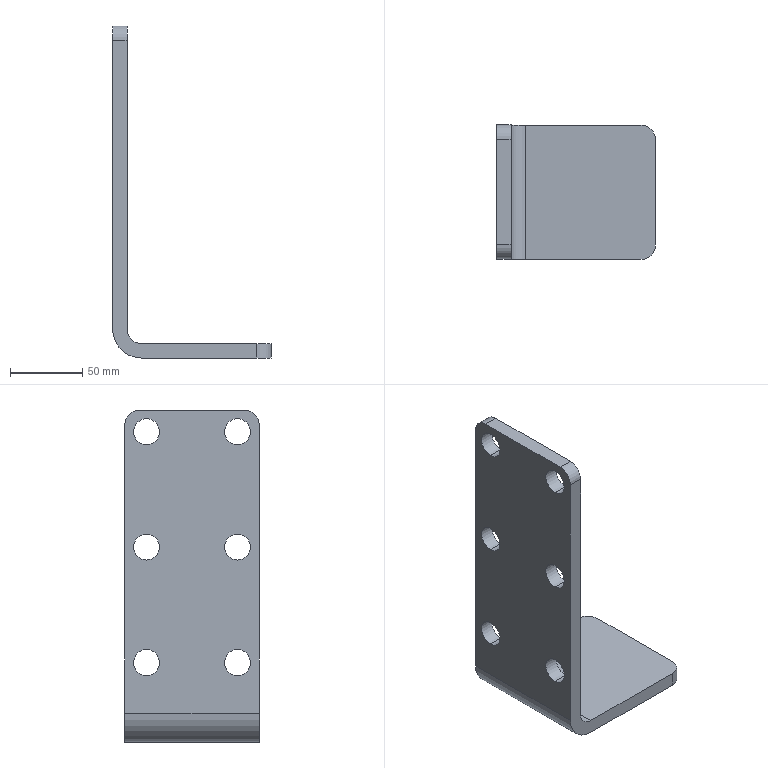Part | STEP file | VD-SYL0380DJ1006_1_5-1_VD-SYL03 | 1 solid | 26 faces | box 110 x 93 x 230 mm | volume 284786 mm3 | cylinder 18 | plane 8 | commonest cylinder face diameters 18 x12 20 x5 40 x1
STEP:
#1=CARTESIAN_POINT('',(0.,-78.,-184.));
#2=VERTEX_POINT('',#1);
#3=CARTESIAN_POINT('',(0.,-78.,-166.));
#4=VERTEX_POINT('',#3);
#5=CARTESIAN_POINT('',(0.,-78.,-175.));
#6=DIRECTION('',(1.,0.,0.));
#7=DIRECTION('',(0.,0.,-1.));
#8=AXIS2_PLACEMENT_3D('',#5,#6,#7);
#9=CIRCLE('',#8,9.);
#10=EDGE_CURVE('',#2,#4,#9,.T.);
#11=ORIENTED_EDGE('',*,*,#10,.F.);
#12=CARTESIAN_POINT('',(10.,-78.,-184.));
#13=VERTEX_POINT('',#12);
#14=CARTESIAN_POINT('',(10.,-78.,-184.));
#15=DIRECTION('',(-1.,0.,0.));
#16=VECTOR('',#15,1000.);
#17=LINE('',#14,#16);
#18=EDGE_CURVE('',#13,#2,#17,.T.);
#19=ORIENTED_EDGE('',*,*,#18,.F.);
#20=CARTESIAN_POINT('',(10.,-78.,-166.));
#21=VERTEX_POINT('',#20);
#22=CARTESIAN_POINT('',(10.,-78.,-175.));
#23=DIRECTION('',(-1.,0.,0.));
#24=DIRECTION('',(0.,0.,1.));
#25=AXIS2_PLACEMENT_3D('',#22,#23,#24);
#26=CIRCLE('',#25,9.);
#27=EDGE_CURVE('',#21,#13,#26,.T.);
#28=ORIENTED_EDGE('',*,*,#27,.F.);
#29=CARTESIAN_POINT('',(10.,-78.,-166.));
#30=DIRECTION('',(-1.,0.,0.));
#31=VECTOR('',#30,1000.);
#32=LINE('',#29,#31);
#33=EDGE_CURVE('',#21,#4,#32,.T.);
#34=ORIENTED_EDGE('',*,*,#33,.T.);
#35=EDGE_LOOP('',(#11,#19,#28,#34));
#36=FACE_OUTER_BOUND('',#35,.T.);
#37=CARTESIAN_POINT('',(5.,-78.,-175.));
#38=DIRECTION('',(1.,0.,0.));
#39=DIRECTION('',(0.,0.,-1.));
#40=AXIS2_PLACEMENT_3D('',#37,#38,#39);
#41=CYLINDRICAL_SURFACE('',#40,9.);
#42=ADVANCED_FACE('',(#36),#41,.F.);
#43=ORIENTED_EDGE('',*,*,#33,.F.);
#44=CARTESIAN_POINT('',(10.,-78.,-175.));
#45=DIRECTION('',(-1.,0.,0.));
#46=DIRECTION('',(0.,0.,-1.));
#47=AXIS2_PLACEMENT_3D('',#44,#45,#46);
#48=CIRCLE('',#47,9.);
#49=EDGE_CURVE('',#13,#21,#48,.T.);
#50=ORIENTED_EDGE('',*,*,#49,.F.);
#51=ORIENTED_EDGE('',*,*,#18,.T.);
#52=CARTESIAN_POINT('',(0.,-78.,-175.));
#53=DIRECTION('',(1.,0.,0.));
#54=DIRECTION('',(0.,0.,1.));
#55=AXIS2_PLACEMENT_3D('',#52,#53,#54);
#56=CIRCLE('',#55,9.);
#57=EDGE_CURVE('',#4,#2,#56,.T.);
#58=ORIENTED_EDGE('',*,*,#57,.F.);
#59=EDGE_LOOP('',(#43,#50,#51,#58));
#60=FACE_OUTER_BOUND('',#59,.T.);
#61=CARTESIAN_POINT('',(5.,-78.,-175.));
#62=DIRECTION('',(1.,0.,0.));
#63=DIRECTION('',(0.,0.,-1.));
#64=AXIS2_PLACEMENT_3D('',#61,#62,#63);
#65=CYLINDRICAL_SURFACE('',#64,9.);
#66=ADVANCED_FACE('',(#60),#65,.F.);
#67=CARTESIAN_POINT('',(0.,-15.,-184.));
#68=VERTEX_POINT('',#67);
#69=CARTESIAN_POINT('',(0.,-15.,-166.));
#70=VERTEX_POINT('',#69);
#71=CARTESIAN_POINT('',(0.,-15.,-175.));
#72=DIRECTION('',(1.,0.,0.));
#73=DIRECTION('',(0.,0.,-1.));
#74=AXIS2_PLACEMENT_3D('',#71,#72,#73);
#75=CIRCLE('',#74,9.);
#76=EDGE_CURVE('',#68,#70,#75,.T.);
#77=ORIENTED_EDGE('',*,*,#76,.F.);
#78=CARTESIAN_POINT('',(10.,-15.,-184.));
#79=VERTEX_POINT('',#78);
#80=CARTESIAN_POINT('',(10.,-15.,-184.));
#81=DIRECTION('',(-1.,0.,0.));
#82=VECTOR('',#81,1000.);
#83=LINE('',#80,#82);
#84=EDGE_CURVE('',#79,#68,#83,.T.);
#85=ORIENTED_EDGE('',*,*,#84,.F.);
#86=CARTESIAN_POINT('',(10.,-15.,-166.));
#87=VERTEX_POINT('',#86);
#88=CARTESIAN_POINT('',(10.,-15.,-175.));
#89=DIRECTION('',(-1.,0.,0.));
#90=DIRECTION('',(0.,0.,1.));
#91=AXIS2_PLACEMENT_3D('',#88,#89,#90);
#92=CIRCLE('',#91,9.);
#93=EDGE_CURVE('',#87,#79,#92,.T.);
#94=ORIENTED_EDGE('',*,*,#93,.F.);
#95=CARTESIAN_POINT('',(10.,-15.,-166.));
#96=DIRECTION('',(-1.,0.,0.));
#97=VECTOR('',#96,1000.);
#98=LINE('',#95,#97);
#99=EDGE_CURVE('',#87,#70,#98,.T.);
#100=ORIENTED_EDGE('',*,*,#99,.T.);
#101=EDGE_LOOP('',(#77,#85,#94,#100));
#102=FACE_OUTER_BOUND('',#101,.T.);
#103=CARTESIAN_POINT('',(5.,-15.,-175.));
#104=DIRECTION('',(1.,0.,0.));
#105=DIRECTION('',(0.,0.,-1.));
#106=AXIS2_PLACEMENT_3D('',#103,#104,#105);
#107=CYLINDRICAL_SURFACE('',#106,9.);
#108=ADVANCED_FACE('',(#102),#107,.F.);
#109=ORIENTED_EDGE('',*,*,#99,.F.);
#110=CARTESIAN_POINT('',(10.,-15.,-175.));
#111=DIRECTION('',(-1.,0.,0.));
#112=DIRECTION('',(0.,0.,-1.));
#113=AXIS2_PLACEMENT_3D('',#110,#111,#112);
#114=CIRCLE('',#113,9.);
#115=EDGE_CURVE('',#79,#87,#114,.T.);
#116=ORIENTED_EDGE('',*,*,#115,.F.);
#117=ORIENTED_EDGE('',*,*,#84,.T.);
#118=CARTESIAN_POINT('',(0.,-15.,-175.));
#119=DIRECTION('',(1.,0.,0.));
#120=DIRECTION('',(0.,0.,1.));
#121=AXIS2_PLACEMENT_3D('',#118,#119,#120);
#122=CIRCLE('',#121,9.);
#123=EDGE_CURVE('',#70,#68,#122,.T.);
#124=ORIENTED_EDGE('',*,*,#123,.F.);
#125=EDGE_LOOP('',(#109,#116,#117,#124));
#126=FACE_OUTER_BOUND('',#125,.T.);
#127=CARTESIAN_POINT('',(5.,-15.,-175.));
#128=DIRECTION('',(1.,0.,0.));
#129=DIRECTION('',(0.,0.,-1.));
#130=AXIS2_PLACEMENT_3D('',#127,#128,#129);
#131=CYLINDRICAL_SURFACE('',#130,9.);
#132=ADVANCED_FACE('',(#126),#131,.F.);
#133=CARTESIAN_POINT('',(0.,-78.,-104.));
#134=VERTEX_POINT('',#133);
#135=CARTESIAN_POINT('',(10.,-78.,-104.));
#136=VERTEX_POINT('',#135);
#137=CARTESIAN_POINT('',(0.,-78.,-104.));
#138=DIRECTION('',(1.,0.,0.));
#139=VECTOR('',#138,1000.);
#140=LINE('',#137,#139);
#141=EDGE_CURVE('',#134,#136,#140,.T.);
#142=ORIENTED_EDGE('',*,*,#141,.F.);
#143=CARTESIAN_POINT('',(0.,-78.,-86.));
#144=VERTEX_POINT('',#143);
#145=CARTESIAN_POINT('',(0.,-78.,-95.));
#146=DIRECTION('',(1.,0.,0.));
#147=DIRECTION('',(0.,0.,1.));
#148=AXIS2_PLACEMENT_3D('',#145,#146,#147);
#149=CIRCLE('',#148,9.);
#150=EDGE_CURVE('',#144,#134,#149,.T.);
#151=ORIENTED_EDGE('',*,*,#150,.F.);
#152=CARTESIAN_POINT('',(10.,-78.,-86.));
#153=VERTEX_POINT('',#152);
#154=CARTESIAN_POINT('',(0.,-78.,-86.));
#155=DIRECTION('',(1.,0.,0.));
#156=VECTOR('',#155,1000.);
#157=LINE('',#154,#156);
#158=EDGE_CURVE('',#144,#153,#157,.T.);
#159=ORIENTED_EDGE('',*,*,#158,.T.);
#160=CARTESIAN_POINT('',(10.,-78.,-95.));
#161=DIRECTION('',(-1.,0.,0.));
#162=DIRECTION('',(0.,0.,-1.));
#163=AXIS2_PLACEMENT_3D('',#160,#161,#162);
#164=CIRCLE('',#163,9.);
#165=EDGE_CURVE('',#136,#153,#164,.T.);
#166=ORIENTED_EDGE('',*,*,#165,.F.);
#167=EDGE_LOOP('',(#142,#151,#159,#166));
#168=FACE_OUTER_BOUND('',#167,.T.);
#169=CARTESIAN_POINT('',(5.,-78.,-95.));
#170=DIRECTION('',(-1.,0.,0.));
#171=DIRECTION('',(0.,0.,1.));
#172=AXIS2_PLACEMENT_3D('',#169,#170,#171);
#173=CYLINDRICAL_SURFACE('',#172,9.);
#174=ADVANCED_FACE('',(#168),#173,.F.);
#175=CARTESIAN_POINT('',(10.,-78.,-95.));
#176=DIRECTION('',(-1.,0.,0.));
#177=DIRECTION('',(0.,0.,1.));
#178=AXIS2_PLACEMENT_3D('',#175,#176,#177);
#179=CIRCLE('',#178,9.);
#180=EDGE_CURVE('',#153,#136,#179,.T.);
#181=ORIENTED_EDGE('',*,*,#180,.F.);
#182=ORIENTED_EDGE('',*,*,#158,.F.);
#183=CARTESIAN_POINT('',(0.,-78.,-95.));
#184=DIRECTION('',(1.,0.,0.));
#185=DIRECTION('',(0.,0.,-1.));
#186=AXIS2_PLACEMENT_3D('',#183,#184,#185);
#187=CIRCLE('',#186,9.);
#188=EDGE_CURVE('',#134,#144,#187,.T.);
#189=ORIENTED_EDGE('',*,*,#188,.F.);
#190=ORIENTED_EDGE('',*,*,#141,.T.);
#191=EDGE_LOOP('',(#181,#182,#189,#190));
#192=FACE_OUTER_BOUND('',#191,.T.);
#193=CARTESIAN_POINT('',(5.,-78.,-95.));
#194=DIRECTION('',(-1.,0.,0.));
#195=DIRECTION('',(0.,0.,1.));
#196=AXIS2_PLACEMENT_3D('',#193,#194,#195);
#197=CYLINDRICAL_SURFACE('',#196,9.);
#198=ADVANCED_FACE('',(#192),#197,.F.);
#199=CARTESIAN_POINT('',(0.,-15.,-104.));
#200=VERTEX_POINT('',#199);
#201=CARTESIAN_POINT('',(10.,-15.,-104.));
#202=VERTEX_POINT('',#201);
#203=CARTESIAN_POINT('',(0.,-15.,-104.));
#204=DIRECTION('',(1.,0.,0.));
#205=VECTOR('',#204,1000.);
#206=LINE('',#203,#205);
#207=EDGE_CURVE('',#200,#202,#206,.T.);
#208=ORIENTED_EDGE('',*,*,#207,.F.);
#209=CARTESIAN_POINT('',(0.,-15.,-86.));
#210=VERTEX_POINT('',#209);
#211=CARTESIAN_POINT('',(0.,-15.,-95.));
#212=DIRECTION('',(1.,0.,0.));
#213=DIRECTION('',(0.,0.,1.));
#214=AXIS2_PLACEMENT_3D('',#211,#212,#213);
#215=CIRCLE('',#214,9.);
#216=EDGE_CURVE('',#210,#200,#215,.T.);
#217=ORIENTED_EDGE('',*,*,#216,.F.);
#218=CARTESIAN_POINT('',(10.,-15.,-86.));
#219=VERTEX_POINT('',#218);
#220=CARTESIAN_POINT('',(0.,-15.,-86.));
#221=DIRECTION('',(1.,0.,0.));
#222=VECTOR('',#221,1000.);
#223=LINE('',#220,#222);
#224=EDGE_CURVE('',#210,#219,#223,.T.);
#225=ORIENTED_EDGE('',*,*,#224,.T.);
#226=CARTESIAN_POINT('',(10.,-15.,-95.));
#227=DIRECTION('',(-1.,0.,0.));
#228=DIRECTION('',(0.,0.,-1.));
#229=AXIS2_PLACEMENT_3D('',#226,#227,#228);
#230=CIRCLE('',#229,9.);
#231=EDGE_CURVE('',#202,#219,#230,.T.);
#232=ORIENTED_EDGE('',*,*,#231,.F.);
#233=EDGE_LOOP('',(#208,#217,#225,#232));
#234=FACE_OUTER_BOUND('',#233,.T.);
#235=CARTESIAN_POINT('',(5.,-15.,-95.));
#236=DIRECTION('',(-1.,0.,0.));
#237=DIRECTION('',(0.,0.,1.));
#238=AXIS2_PLACEMENT_3D('',#235,#236,#237);
#239=CYLINDRICAL_SURFACE('',#238,9.);
#240=ADVANCED_FACE('',(#234),#239,.F.);
#241=CARTESIAN_POINT('',(10.,-15.,-95.));
#242=DIRECTION('',(-1.,0.,0.));
#243=DIRECTION('',(0.,0.,1.));
#244=AXIS2_PLACEMENT_3D('',#241,#242,#243);
#245=CIRCLE('',#244,9.);
#246=EDGE_CURVE('',#219,#202,#245,.T.);
#247=ORIENTED_EDGE('',*,*,#246,.F.);
#248=ORIENTED_EDGE('',*,*,#224,.F.);
#249=CARTESIAN_POINT('',(0.,-15.,-95.));
#250=DIRECTION('',(1.,0.,0.));
#251=DIRECTION('',(0.,0.,-1.));
#252=AXIS2_PLACEMENT_3D('',#249,#250,#251);
#253=CIRCLE('',#252,9.);
#254=EDGE_CURVE('',#200,#210,#253,.T.);
#255=ORIENTED_EDGE('',*,*,#254,.F.);
#256=ORIENTED_EDGE('',*,*,#207,.T.);
#257=EDGE_LOOP('',(#247,#248,#255,#256));
#258=FACE_OUTER_BOUND('',#257,.T.);
#259=CARTESIAN_POINT('',(5.,-15.,-95.));
#260=DIRECTION('',(-1.,0.,0.));
#261=DIRECTION('',(0.,0.,1.));
#262=AXIS2_PLACEMENT_3D('',#259,#260,#261);
#263=CYLINDRICAL_SURFACE('',#262,9.);
#264=ADVANCED_FACE('',(#258),#263,.F.);
#265=CARTESIAN_POINT('',(0.,-78.,-24.));
#266=VERTEX_POINT('',#265);
#267=CARTESIAN_POINT('',(10.,-78.,-24.));
#268=VERTEX_POINT('',#267);
#269=CARTESIAN_POINT('',(0.,-78.,-24.));
#270=DIRECTION('',(1.,0.,0.));
#271=VECTOR('',#270,1000.);
#272=LINE('',#269,#271);
#273=EDGE_CURVE('',#266,#268,#272,.T.);
#274=ORIENTED_EDGE('',*,*,#273,.F.);
#275=CARTESIAN_POINT('',(0.,-78.,-6.));
#276=VERTEX_POINT('',#275);
#277=CARTESIAN_POINT('',(0.,-78.,-15.));
#278=DIRECTION('',(1.,0.,0.));
#279=DIRECTION('',(0.,0.,1.));
#280=AXIS2_PLACEMENT_3D('',#277,#278,#279);
#281=CIRCLE('',#280,9.);
#282=EDGE_CURVE('',#276,#266,#281,.T.);
#283=ORIENTED_EDGE('',*,*,#282,.F.);
#284=CARTESIAN_POINT('',(10.,-78.,-6.));
#285=VERTEX_POINT('',#284);
#286=CARTESIAN_POINT('',(0.,-78.,-6.));
#287=DIRECTION('',(1.,0.,0.));
#288=VECTOR('',#287,1000.);
#289=LINE('',#286,#288);
#290=EDGE_CURVE('',#276,#285,#289,.T.);
#291=ORIENTED_EDGE('',*,*,#290,.T.);
#292=CARTESIAN_POINT('',(10.,-78.,-15.));
#293=DIRECTION('',(-1.,0.,0.));
#294=DIRECTION('',(0.,0.,-1.));
#295=AXIS2_PLACEMENT_3D('',#292,#293,#294);
#296=CIRCLE('',#295,9.);
#297=EDGE_CURVE('',#268,#285,#296,.T.);
#298=ORIENTED_EDGE('',*,*,#297,.F.);
#299=EDGE_LOOP('',(#274,#283,#291,#298));
#300=FACE_OUTER_BOUND('',#299,.T.);
#301=CARTESIAN_POINT('',(5.,-78.,-15.));
#302=DIRECTION('',(-1.,0.,0.));
#303=DIRECTION('',(0.,0.,1.));
#304=AXIS2_PLACEMENT_3D('',#301,#302,#303);
#305=CYLINDRICAL_SURFACE('',#304,9.);
#306=ADVANCED_FACE('',(#300),#305,.F.);
#307=CARTESIAN_POINT('',(10.,-78.,-15.));
#308=DIRECTION('',(-1.,0.,0.));
#309=DIRECTION('',(0.,0.,1.));
#310=AXIS2_PLACEMENT_3D('',#307,#308,#309);
#311=CIRCLE('',#310,9.);
#312=EDGE_CURVE('',#285,#268,#311,.T.);
#313=ORIENTED_EDGE('',*,*,#312,.F.);
#314=ORIENTED_EDGE('',*,*,#290,.F.);
#315=CARTESIAN_POINT('',(0.,-78.,-15.));
#316=DIRECTION('',(1.,0.,0.));
#317=DIRECTION('',(0.,0.,-1.));
#318=AXIS2_PLACEMENT_3D('',#315,#316,#317);
#319=CIRCLE('',#318,9.);
#320=EDGE_CURVE('',#266,#276,#319,.T.);
#321=ORIENTED_EDGE('',*,*,#320,.F.);
#322=ORIENTED_EDGE('',*,*,#273,.T.);
#323=EDGE_LOOP('',(#313,#314,#321,#322));
#324=FACE_OUTER_BOUND('',#323,.T.);
#325=CARTESIAN_POINT('',(5.,-78.,-15.));
#326=DIRECTION('',(-1.,0.,0.));
#327=DIRECTION('',(0.,0.,1.));
#328=AXIS2_PLACEMENT_3D('',#325,#326,#327);
#329=CYLINDRICAL_SURFACE('',#328,9.);
#330=ADVANCED_FACE('',(#324),#329,.F.);
#331=CARTESIAN_POINT('',(0.,-15.,-24.));
#332=VERTEX_POINT('',#331);
#333=CARTESIAN_POINT('',(10.,-15.,-24.));
#334=VERTEX_POINT('',#333);
#335=CARTESIAN_POINT('',(0.,-15.,-24.));
#336=DIRECTION('',(1.,0.,0.));
#337=VECTOR('',#336,1000.);
#338=LINE('',#335,#337);
#339=EDGE_CURVE('',#332,#334,#338,.T.);
#340=ORIENTED_EDGE('',*,*,#339,.F.);
#341=CARTESIAN_POINT('',(0.,-15.,-6.));
#342=VERTEX_POINT('',#341);
#343=CARTESIAN_POINT('',(0.,-15.,-15.));
#344=DIRECTION('',(1.,0.,0.));
#345=DIRECTION('',(0.,0.,1.));
#346=AXIS2_PLACEMENT_3D('',#343,#344,#345);
#347=CIRCLE('',#346,9.);
#348=EDGE_CURVE('',#342,#332,#347,.T.);
#349=ORIENTED_EDGE('',*,*,#348,.F.);
#350=CARTESIAN_POINT('',(10.,-15.,-6.));
#351=VERTEX_POINT('',#350);
#352=CARTESIAN_POINT('',(0.,-15.,-6.));
#353=DIRECTION('',(1.,0.,0.));
#354=VECTOR('',#353,1000.);
#355=LINE('',#352,#354);
#356=EDGE_CURVE('',#342,#351,#355,.T.);
#357=ORIENTED_EDGE('',*,*,#356,.T.);
#358=CARTESIAN_POINT('',(10.,-15.,-15.));
#359=DIRECTION('',(-1.,0.,0.));
#360=DIRECTION('',(0.,0.,-1.));
#361=AXIS2_PLACEMENT_3D('',#358,#359,#360);
#362=CIRCLE('',#361,9.);
#363=EDGE_CURVE('',#334,#351,#362,.T.);
#364=ORIENTED_EDGE('',*,*,#363,.F.);
#365=EDGE_LOOP('',(#340,#349,#357,#364));
#366=FACE_OUTER_BOUND('',#365,.T.);
#367=CARTESIAN_POINT('',(5.,-15.,-15.));
#368=DIRECTION('',(-1.,0.,0.));
#369=DIRECTION('',(0.,0.,1.));
#370=AXIS2_PLACEMENT_3D('',#367,#368,#369);
#371=CYLINDRICAL_SURFACE('',#370,9.);
#372=ADVANCED_FACE('',(#366),#371,.F.);
#373=CARTESIAN_POINT('',(10.,-15.,-15.));
#374=DIRECTION('',(-1.,0.,0.));
#375=DIRECTION('',(0.,0.,1.));
#376=AXIS2_PLACEMENT_3D('',#373,#374,#375);
#377=CIRCLE('',#376,9.);
#378=EDGE_CURVE('',#351,#334,#377,.T.);
#379=ORIENTED_EDGE('',*,*,#378,.F.);
#380=ORIENTED_EDGE('',*,*,#356,.F.);
#381=CARTESIAN_POINT('',(0.,-15.,-15.));
#382=DIRECTION('',(1.,0.,0.));
#383=DIRECTION('',(0.,0.,-1.));
#384=AXIS2_PLACEMENT_3D('',#381,#382,#383);
#385=CIRCLE('',#384,9.);
#386=EDGE_CURVE('',#332,#342,#385,.T.);
#387=ORIENTED_EDGE('',*,*,#386,.F.);
#388=ORIENTED_EDGE('',*,*,#339,.T.);
#389=EDGE_LOOP('',(#379,#380,#387,#388));
#390=FACE_OUTER_BOUND('',#389,.T.);
#391=CARTESIAN_POINT('',(5.,-15.,-15.));
#392=DIRECTION('',(-1.,0.,0.));
#393=DIRECTION('',(0.,0.,1.));
#394=AXIS2_PLACEMENT_3D('',#391,#392,#393);
#395=CYLINDRICAL_SURFACE('',#394,9.);
#396=ADVANCED_FACE('',(#390),#395,.F.);
#397=CARTESIAN_POINT('',(100.,0.,-230.));
#398=VERTEX_POINT('',#397);
#399=CARTESIAN_POINT('',(110.,-10.,-230.));
#400=VERTEX_POINT('',#399);
#401=CARTESIAN_POINT('',(100.,-10.,-230.));
#402=DIRECTION('',(0.,0.,-1.));
#403=DIRECTION('',(0.,1.,0.));
#404=AXIS2_PLACEMENT_3D('',#401,#402,#403);
#405=CIRCLE('',#404,10.);
#406=EDGE_CURVE('',#398,#400,#405,.T.);
#407=ORIENTED_EDGE('',*,*,#406,.F.);
#408=CARTESIAN_POINT('',(100.,0.,-220.));
#409=VERTEX_POINT('',#408);
#410=CARTESIAN_POINT('',(100.,0.,-230.));
#411=DIRECTION('',(0.,0.,1.));
#412=VECTOR('',#411,1000.);
#413=LINE('',#410,#412);
#414=EDGE_CURVE('',#398,#409,#413,.T.);
#415=ORIENTED_EDGE('',*,*,#414,.T.);
#416=CARTESIAN_POINT('',(110.,-10.,-220.));
#417=VERTEX_POINT('',#416);
#418=CARTESIAN_POINT('',(100.,-10.,-220.));
#419=DIRECTION('',(0.,0.,1.));
#420=DIRECTION('',(1.,0.,0.));
#421=AXIS2_PLACEMENT_3D('',#418,#419,#420);
#422=CIRCLE('',#421,10.);
#423=EDGE_CURVE('',#417,#409,#422,.T.);
#424=ORIENTED_EDGE('',*,*,#423,.F.);
#425=CARTESIAN_POINT('',(110.,-10.,-220.));
#426=DIRECTION('',(0.,0.,-1.));
#427=VECTOR('',#426,1000.);
#428=LINE('',#425,#427);
#429=EDGE_CURVE('',#417,#400,#428,.T.);
#430=ORIENTED_EDGE('',*,*,#429,.T.);
#431=EDGE_LOOP('',(#407,#415,#424,#430));
#432=FACE_OUTER_BOUND('',#431,.T.);
#433=CARTESIAN_POINT('',(100.,-10.,-225.));
#434=DIRECTION('',(0.,0.,-1.));
#435=DIRECTION('',(-1.,0.,0.));
#436=AXIS2_PLACEMENT_3D('',#433,#434,#435);
#437=CYLINDRICAL_SURFACE('',#436,10.);
#438=ADVANCED_FACE('',(#432),#437,.T.);
#439=CARTESIAN_POINT('',(0.,-10.,0.));
#440=VERTEX_POINT('',#439);
#441=CARTESIAN_POINT('',(0.,0.,-10.));
#442=VERTEX_POINT('',#441);
#443=CARTESIAN_POINT('',(0.,-10.,-10.));
#444=DIRECTION('',(-1.,0.,0.));
#445=DIRECTION('',(0.,0.,1.));
#446=AXIS2_PLACEMENT_3D('',#443,#444,#445);
#447=CIRCLE('',#446,10.);
#448=EDGE_CURVE('',#440,#442,#447,.T.);
#449=ORIENTED_EDGE('',*,*,#448,.F.);
#450=CARTESIAN_POINT('',(10.,-10.,0.));
#451=VERTEX_POINT('',#450);
#452=CARTESIAN_POINT('',(0.,-10.,0.));
#453=DIRECTION('',(1.,0.,0.));
#454=VECTOR('',#453,1000.);
#455=LINE('',#452,#454);
#456=EDGE_CURVE('',#440,#451,#455,.T.);
#457=ORIENTED_EDGE('',*,*,#456,.T.);
#458=CARTESIAN_POINT('',(10.,0.,-10.));
#459=VERTEX_POINT('',#458);
#460=CARTESIAN_POINT('',(10.,-10.,-10.));
#461=DIRECTION('',(1.,0.,0.));
#462=DIRECTION('',(0.,1.,0.));
#463=AXIS2_PLACEMENT_3D('',#460,#461,#462);
#464=CIRCLE('',#463,10.);
#465=EDGE_CURVE('',#459,#451,#464,.T.);
#466=ORIENTED_EDGE('',*,*,#465,.F.);
#467=CARTESIAN_POINT('',(10.,0.,-10.));
#468=DIRECTION('',(-1.,0.,0.));
#469=VECTOR('',#468,1000.);
#470=LINE('',#467,#469);
#471=EDGE_CURVE('',#459,#442,#470,.T.);
#472=ORIENTED_EDGE('',*,*,#471,.T.);
#473=EDGE_LOOP('',(#449,#457,#466,#472));
#474=FACE_OUTER_BOUND('',#473,.T.);
#475=CARTESIAN_POINT('',(5.,-10.,-10.));
#476=DIRECTION('',(1.,0.,0.));
#477=DIRECTION('',(0.,0.,-1.));
#478=AXIS2_PLACEMENT_3D('',#475,#476,#477);
#479=CYLINDRICAL_SURFACE('',#478,10.);
#480=ADVANCED_FACE('',(#474),#479,.T.);
#481=CARTESIAN_POINT('',(10.,0.,-210.));
#482=VERTEX_POINT('',#481);
#483=CARTESIAN_POINT('',(20.,0.,-220.));
#484=VERTEX_POINT('',#483);
#485=CARTESIAN_POINT('',(20.,0.,-210.));
#486=DIRECTION('',(0.,-1.,0.));
#487=DIRECTION('',(-1.,0.,0.));
#488=AXIS2_PLACEMENT_3D('',#485,#486,#487);
#489=CIRCLE('',#488,10.);
#490=EDGE_CURVE('',#482,#484,#489,.T.);
#491=ORIENTED_EDGE('',*,*,#490,.T.);
#492=CARTESIAN_POINT('',(20.,0.,-220.));
#493=DIRECTION('',(1.,0.,0.));
#494=VECTOR('',#493,1000.);
#495=LINE('',#492,#494);
#496=EDGE_CURVE('',#484,#409,#495,.T.);
#497=ORIENTED_EDGE('',*,*,#496,.T.);
#498=ORIENTED_EDGE('',*,*,#414,.F.);
#499=CARTESIAN_POINT('',(20.,0.,-230.));
#500=VERTEX_POINT('',#499);
#501=CARTESIAN_POINT('',(100.,0.,-230.));
#502=DIRECTION('',(-1.,0.,0.));
#503=VECTOR('',#502,1000.);
#504=LINE('',#501,#503);
#505=EDGE_CURVE('',#398,#500,#504,.T.);
#506=ORIENTED_EDGE('',*,*,#505,.T.);
#507=CARTESIAN_POINT('',(0.,0.,-210.));
#508=VERTEX_POINT('',#507);
#509=CARTESIAN_POINT('',(20.,0.,-210.));
#510=DIRECTION('',(0.,1.,0.));
#511=DIRECTION('',(0.,0.,-1.));
#512=AXIS2_PLACEMENT_3D('',#509,#510,#511);
#513=CIRCLE('',#512,20.);
#514=EDGE_CURVE('',#500,#508,#513,.T.);
#515=ORIENTED_EDGE('',*,*,#514,.T.);
#516=CARTESIAN_POINT('',(0.,0.,-10.));
#517=DIRECTION('',(0.,0.,-1.));
#518=VECTOR('',#517,1000.);
#519=LINE('',#516,#518);
#520=EDGE_CURVE('',#442,#508,#519,.T.);
#521=ORIENTED_EDGE('',*,*,#520,.F.);
#522=ORIENTED_EDGE('',*,*,#471,.F.);
#523=CARTESIAN_POINT('',(10.,0.,-10.));
#524=DIRECTION('',(0.,0.,-1.));
#525=VECTOR('',#524,1000.);
#526=LINE('',#523,#525);
#527=EDGE_CURVE('',#459,#482,#526,.T.);
#528=ORIENTED_EDGE('',*,*,#527,.T.);
#529=EDGE_LOOP('',(#491,#497,#498,#506,#515,#521,#522,#528));
#530=FACE_OUTER_BOUND('',#529,.T.);
#531=CARTESIAN_POINT('',(5.,0.,-110.));
#532=DIRECTION('',(0.,-1.,0.));
#533=DIRECTION('',(0.,0.,-1.));
#534=AXIS2_PLACEMENT_3D('',#531,#532,#533);
#535=PLANE('',#534);
#536=ADVANCED_FACE('',(#530),#535,.F.);
#537=CARTESIAN_POINT('',(10.,-93.,-210.));
#538=VERTEX_POINT('',#537);
#539=CARTESIAN_POINT('',(10.,0.,-210.));
#540=DIRECTION('',(0.,-1.,0.));
#541=VECTOR('',#540,1000.);
#542=LINE('',#539,#541);
#543=EDGE_CURVE('',#482,#538,#542,.T.);
#544=ORIENTED_EDGE('',*,*,#543,.T.);
#545=CARTESIAN_POINT('',(20.,-93.,-220.));
#546=VERTEX_POINT('',#545);
#547=CARTESIAN_POINT('',(20.,-93.,-210.));
#548=DIRECTION('',(0.,1.,0.));
#549=DIRECTION('',(0.,0.,-1.));
#550=AXIS2_PLACEMENT_3D('',#547,#548,#549);
#551=CIRCLE('',#550,10.);
#552=EDGE_CURVE('',#546,#538,#551,.T.);
#553=ORIENTED_EDGE('',*,*,#552,.F.);
#554=CARTESIAN_POINT('',(20.,-93.,-220.));
#555=DIRECTION('',(0.,1.,0.));
#556=VECTOR('',#555,1000.);
#557=LINE('',#554,#556);
#558=EDGE_CURVE('',#546,#484,#557,.T.);
#559=ORIENTED_EDGE('',*,*,#558,.T.);
#560=ORIENTED_EDGE('',*,*,#490,.F.);
#561=EDGE_LOOP('',(#544,#553,#559,#560));
#562=FACE_OUTER_BOUND('',#561,.T.);
#563=CARTESIAN_POINT('',(20.,121.235,-210.));
#564=DIRECTION('',(0.,-1.,0.));
#565=DIRECTION('',(0.,0.,-1.));
#566=AXIS2_PLACEMENT_3D('',#563,#564,#565);
#567=CYLINDRICAL_SURFACE('',#566,10.);
#568=ADVANCED_FACE('',(#562),#567,.F.);
#569=CARTESIAN_POINT('',(110.,-83.,-220.));
#570=VERTEX_POINT('',#569);
#571=CARTESIAN_POINT('',(110.,-10.,-220.));
#572=DIRECTION('',(0.,-1.,0.));
#573=VECTOR('',#572,1000.);
#574=LINE('',#571,#573);
#575=EDGE_CURVE('',#417,#570,#574,.T.);
#576=ORIENTED_EDGE('',*,*,#575,.F.);
#577=ORIENTED_EDGE('',*,*,#423,.T.);
#578=ORIENTED_EDGE('',*,*,#496,.F.);
#579=ORIENTED_EDGE('',*,*,#558,.F.);
#580=CARTESIAN_POINT('',(100.,-93.,-220.));
#581=VERTEX_POINT('',#580);
#582=CARTESIAN_POINT('',(100.,-93.,-220.));
#583=DIRECTION('',(-1.,0.,0.));
#584=VECTOR('',#583,1000.);
#585=LINE('',#582,#584);
#586=EDGE_CURVE('',#581,#546,#585,.T.);
#587=ORIENTED_EDGE('',*,*,#586,.F.);
#588=CARTESIAN_POINT('',(100.,-83.,-220.));
#589=DIRECTION('',(0.,0.,1.));
#590=DIRECTION('',(0.,-1.,0.));
#591=AXIS2_PLACEMENT_3D('',#588,#589,#590);
#592=CIRCLE('',#591,10.);
#593=EDGE_CURVE('',#581,#570,#592,.T.);
#594=ORIENTED_EDGE('',*,*,#593,.T.);
#595=EDGE_LOOP('',(#576,#577,#578,#579,#587,#594));
#596=FACE_OUTER_BOUND('',#595,.T.);
#597=CARTESIAN_POINT('',(0.,-93.,-220.));
#598=DIRECTION('',(0.,0.,-1.));
#599=DIRECTION('',(0.,-1.,0.));
#600=AXIS2_PLACEMENT_3D('',#597,#598,#599);
#601=PLANE('',#600);
#602=ADVANCED_FACE('',(#596),#601,.F.);
#603=CARTESIAN_POINT('',(110.,-83.,-230.));
#604=VERTEX_POINT('',#603);
#605=CARTESIAN_POINT('',(110.,-83.,-230.));
#606=DIRECTION('',(0.,0.,1.));
#607=VECTOR('',#606,1000.);
#608=LINE('',#605,#607);
#609=EDGE_CURVE('',#604,#570,#608,.T.);
#610=ORIENTED_EDGE('',*,*,#609,.F.);
#611=CARTESIAN_POINT('',(110.,-83.,-230.));
#612=DIRECTION('',(0.,1.,0.));
#613=VECTOR('',#612,1000.);
#614=LINE('',#611,#613);
#615=EDGE_CURVE('',#604,#400,#614,.T.);
#616=ORIENTED_EDGE('',*,*,#615,.T.);
#617=ORIENTED_EDGE('',*,*,#429,.F.);
#618=ORIENTED_EDGE('',*,*,#575,.T.);
#619=EDGE_LOOP('',(#610,#616,#617,#618));
#620=FACE_OUTER_BOUND('',#619,.T.);
#621=CARTESIAN_POINT('',(110.,-46.5,-225.));
#622=DIRECTION('',(-1.,0.,0.));
#623=DIRECTION('',(0.,0.,1.));
#624=AXIS2_PLACEMENT_3D('',#621,#622,#623);
#625=PLANE('',#624);
#626=ADVANCED_FACE('',(#620),#625,.F.);
#627=CARTESIAN_POINT('',(20.,-93.,-230.));
#628=VERTEX_POINT('',#627);
#629=CARTESIAN_POINT('',(20.,0.,-230.));
#630=DIRECTION('',(0.,-1.,0.));
#631=VECTOR('',#630,1000.);
#632=LINE('',#629,#631);
#633=EDGE_CURVE('',#500,#628,#632,.T.);
#634=ORIENTED_EDGE('',*,*,#633,.F.);
#635=ORIENTED_EDGE('',*,*,#505,.F.);
#636=ORIENTED_EDGE('',*,*,#406,.T.);
#637=ORIENTED_EDGE('',*,*,#615,.F.);
#638=CARTESIAN_POINT('',(100.,-93.,-230.));
#639=VERTEX_POINT('',#638);
#640=CARTESIAN_POINT('',(100.,-83.,-230.));
#641=DIRECTION('',(0.,0.,-1.));
#642=DIRECTION('',(1.,0.,0.));
#643=AXIS2_PLACEMENT_3D('',#640,#641,#642);
#644=CIRCLE('',#643,10.);
#645=EDGE_CURVE('',#604,#639,#644,.T.);
#646=ORIENTED_EDGE('',*,*,#645,.T.);
#647=CARTESIAN_POINT('',(20.,-93.,-230.));
#648=DIRECTION('',(1.,0.,0.));
#649=VECTOR('',#648,1000.);
#650=LINE('',#647,#649);
#651=EDGE_CURVE('',#628,#639,#650,.T.);
#652=ORIENTED_EDGE('',*,*,#651,.F.);
#653=EDGE_LOOP('',(#634,#635,#636,#637,#646,#652));
#654=FACE_OUTER_BOUND('',#653,.T.);
#655=CARTESIAN_POINT('',(0.,-93.,-230.));
#656=DIRECTION('',(0.,0.,-1.));
#657=DIRECTION('',(0.,-1.,0.));
#658=AXIS2_PLACEMENT_3D('',#655,#656,#657);
#659=PLANE('',#658);
#660=ADVANCED_FACE('',(#654),#659,.T.);
#661=CARTESIAN_POINT('',(0.,-93.,-210.));
#662=VERTEX_POINT('',#661);
#663=CARTESIAN_POINT('',(20.,-93.,-210.));
#664=DIRECTION('',(0.,-1.,0.));
#665=DIRECTION('',(-1.,0.,0.));
#666=AXIS2_PLACEMENT_3D('',#663,#664,#665);
#667=CIRCLE('',#666,20.);
#668=EDGE_CURVE('',#662,#628,#667,.T.);
#669=ORIENTED_EDGE('',*,*,#668,.F.);
#670=CARTESIAN_POINT('',(0.,-93.,-210.));
#671=DIRECTION('',(0.,1.,0.));
#672=VECTOR('',#671,1000.);
#673=LINE('',#670,#672);
#674=EDGE_CURVE('',#662,#508,#673,.T.);
#675=ORIENTED_EDGE('',*,*,#674,.T.);
#676=ORIENTED_EDGE('',*,*,#514,.F.);
#677=ORIENTED_EDGE('',*,*,#633,.T.);
#678=EDGE_LOOP('',(#669,#675,#676,#677));
#679=FACE_OUTER_BOUND('',#678,.T.);
#680=CARTESIAN_POINT('',(20.,121.235,-210.));
#681=DIRECTION('',(0.,-1.,0.));
#682=DIRECTION('',(0.,0.,-1.));
#683=AXIS2_PLACEMENT_3D('',#680,#681,#682);
#684=CYLINDRICAL_SURFACE('',#683,20.);
#685=ADVANCED_FACE('',(#679),#684,.T.);
#686=ORIENTED_EDGE('',*,*,#10,.T.);
#687=ORIENTED_EDGE('',*,*,#57,.T.);
#688=EDGE_LOOP('',(#686,#687));
#689=FACE_BOUND('',#688,.T.);
#690=ORIENTED_EDGE('',*,*,#76,.T.);
#691=ORIENTED_EDGE('',*,*,#123,.T.);
#692=EDGE_LOOP('',(#690,#691));
#693=FACE_BOUND('',#692,.T.);
#694=ORIENTED_EDGE('',*,*,#150,.T.);
#695=ORIENTED_EDGE('',*,*,#188,.T.);
#696=EDGE_LOOP('',(#694,#695));
#697=FACE_BOUND('',#696,.T.);
#698=ORIENTED_EDGE('',*,*,#216,.T.);
#699=ORIENTED_EDGE('',*,*,#254,.T.);
#700=EDGE_LOOP('',(#698,#699));
#701=FACE_BOUND('',#700,.T.);
#702=ORIENTED_EDGE('',*,*,#282,.T.);
#703=ORIENTED_EDGE('',*,*,#320,.T.);
#704=EDGE_LOOP('',(#702,#703));
#705=FACE_BOUND('',#704,.T.);
#706=ORIENTED_EDGE('',*,*,#348,.T.);
#707=ORIENTED_EDGE('',*,*,#386,.T.);
#708=EDGE_LOOP('',(#706,#707));
#709=FACE_BOUND('',#708,.T.);
#710=CARTESIAN_POINT('',(0.,-83.,0.));
#711=VERTEX_POINT('',#710);
#712=CARTESIAN_POINT('',(0.,-83.,0.));
#713=DIRECTION('',(0.,1.,0.));
#714=VECTOR('',#713,1000.);
#715=LINE('',#712,#714);
#716=EDGE_CURVE('',#711,#440,#715,.T.);
#717=ORIENTED_EDGE('',*,*,#716,.T.);
#718=ORIENTED_EDGE('',*,*,#448,.T.);
#719=ORIENTED_EDGE('',*,*,#520,.T.);
#720=ORIENTED_EDGE('',*,*,#674,.F.);
#721=CARTESIAN_POINT('',(0.,-93.,-10.));
#722=VERTEX_POINT('',#721);
#723=CARTESIAN_POINT('',(0.,-93.,-210.));
#724=DIRECTION('',(0.,0.,1.));
#725=VECTOR('',#724,1000.);
#726=LINE('',#723,#725);
#727=EDGE_CURVE('',#662,#722,#726,.T.);
#728=ORIENTED_EDGE('',*,*,#727,.T.);
#729=CARTESIAN_POINT('',(0.,-83.,-10.));
#730=DIRECTION('',(-1.,0.,0.));
#731=DIRECTION('',(0.,-1.,0.));
#732=AXIS2_PLACEMENT_3D('',#729,#730,#731);
#733=CIRCLE('',#732,10.);
#734=EDGE_CURVE('',#722,#711,#733,.T.);
#735=ORIENTED_EDGE('',*,*,#734,.T.);
#736=EDGE_LOOP('',(#717,#718,#719,#720,#728,#735));
#737=FACE_OUTER_BOUND('',#736,.T.);
#738=CARTESIAN_POINT('',(0.,0.,0.));
#739=DIRECTION('',(1.,0.,0.));
#740=DIRECTION('',(0.,1.,0.));
#741=AXIS2_PLACEMENT_3D('',#738,#739,#740);
#742=PLANE('',#741);
#743=ADVANCED_FACE('',(#689,#693,#697,#701,#705,#709,#737),#742,.F.);
#744=ORIENTED_EDGE('',*,*,#456,.F.);
#745=ORIENTED_EDGE('',*,*,#716,.F.);
#746=CARTESIAN_POINT('',(10.,-83.,0.));
#747=VERTEX_POINT('',#746);
#748=CARTESIAN_POINT('',(10.,-83.,0.));
#749=DIRECTION('',(-1.,0.,0.));
#750=VECTOR('',#749,1000.);
#751=LINE('',#748,#750);
#752=EDGE_CURVE('',#747,#711,#751,.T.);
#753=ORIENTED_EDGE('',*,*,#752,.F.);
#754=CARTESIAN_POINT('',(10.,-83.,0.));
#755=DIRECTION('',(0.,1.,0.));
#756=VECTOR('',#755,1000.);
#757=LINE('',#754,#756);
#758=EDGE_CURVE('',#747,#451,#757,.T.);
#759=ORIENTED_EDGE('',*,*,#758,.T.);
#760=EDGE_LOOP('',(#744,#745,#753,#759));
#761=FACE_OUTER_BOUND('',#760,.T.);
#762=CARTESIAN_POINT('',(5.,-46.5,0.));
#763=DIRECTION('',(0.,0.,-1.));
#764=DIRECTION('',(0.,-1.,0.));
#765=AXIS2_PLACEMENT_3D('',#762,#763,#764);
#766=PLANE('',#765);
#767=ADVANCED_FACE('',(#761),#766,.F.);
#768=ORIENTED_EDGE('',*,*,#734,.F.);
#769=CARTESIAN_POINT('',(10.,-93.,-10.));
#770=VERTEX_POINT('',#769);
#771=CARTESIAN_POINT('',(0.,-93.,-10.));
#772=DIRECTION('',(1.,0.,0.));
#773=VECTOR('',#772,1000.);
#774=LINE('',#771,#773);
#775=EDGE_CURVE('',#722,#770,#774,.T.);
#776=ORIENTED_EDGE('',*,*,#775,.T.);
#777=CARTESIAN_POINT('',(10.,-83.,-10.));
#778=DIRECTION('',(1.,0.,0.));
#779=DIRECTION('',(0.,0.,1.));
#780=AXIS2_PLACEMENT_3D('',#777,#778,#779);
#781=CIRCLE('',#780,10.);
#782=EDGE_CURVE('',#747,#770,#781,.T.);
#783=ORIENTED_EDGE('',*,*,#782,.F.);
#784=ORIENTED_EDGE('',*,*,#752,.T.);
#785=EDGE_LOOP('',(#768,#776,#783,#784));
#786=FACE_OUTER_BOUND('',#785,.T.);
#787=CARTESIAN_POINT('',(5.,-83.,-10.));
#788=DIRECTION('',(1.,0.,0.));
#789=DIRECTION('',(0.,0.,-1.));
#790=AXIS2_PLACEMENT_3D('',#787,#788,#789);
#791=CYLINDRICAL_SURFACE('',#790,10.);
#792=ADVANCED_FACE('',(#786),#791,.T.);
#793=ORIENTED_EDGE('',*,*,#27,.T.);
#794=ORIENTED_EDGE('',*,*,#49,.T.);
#795=EDGE_LOOP('',(#793,#794));
#796=FACE_BOUND('',#795,.T.);
#797=ORIENTED_EDGE('',*,*,#93,.T.);
#798=ORIENTED_EDGE('',*,*,#115,.T.);
#799=EDGE_LOOP('',(#797,#798));
#800=FACE_BOUND('',#799,.T.);
#801=ORIENTED_EDGE('',*,*,#165,.T.);
#802=ORIENTED_EDGE('',*,*,#180,.T.);
#803=EDGE_LOOP('',(#801,#802));
#804=FACE_BOUND('',#803,.T.);
#805=ORIENTED_EDGE('',*,*,#231,.T.);
#806=ORIENTED_EDGE('',*,*,#246,.T.);
#807=EDGE_LOOP('',(#805,#806));
#808=FACE_BOUND('',#807,.T.);
#809=ORIENTED_EDGE('',*,*,#297,.T.);
#810=ORIENTED_EDGE('',*,*,#312,.T.);
#811=EDGE_LOOP('',(#809,#810));
#812=FACE_BOUND('',#811,.T.);
#813=ORIENTED_EDGE('',*,*,#363,.T.);
#814=ORIENTED_EDGE('',*,*,#378,.T.);
#815=EDGE_LOOP('',(#813,#814));
#816=FACE_BOUND('',#815,.T.);
#817=ORIENTED_EDGE('',*,*,#543,.F.);
#818=ORIENTED_EDGE('',*,*,#527,.F.);
#819=ORIENTED_EDGE('',*,*,#465,.T.);
#820=ORIENTED_EDGE('',*,*,#758,.F.);
#821=ORIENTED_EDGE('',*,*,#782,.T.);
#822=CARTESIAN_POINT('',(10.,-93.,-210.));
#823=DIRECTION('',(0.,0.,1.));
#824=VECTOR('',#823,1000.);
#825=LINE('',#822,#824);
#826=EDGE_CURVE('',#538,#770,#825,.T.);
#827=ORIENTED_EDGE('',*,*,#826,.F.);
#828=EDGE_LOOP('',(#817,#818,#819,#820,#821,#827));
#829=FACE_OUTER_BOUND('',#828,.T.);
#830=CARTESIAN_POINT('',(10.,0.,0.));
#831=DIRECTION('',(1.,0.,0.));
#832=DIRECTION('',(0.,1.,0.));
#833=AXIS2_PLACEMENT_3D('',#830,#831,#832);
#834=PLANE('',#833);
#835=ADVANCED_FACE('',(#796,#800,#804,#808,#812,#816,#829),#834,.T.);
#836=ORIENTED_EDGE('',*,*,#775,.F.);
#837=ORIENTED_EDGE('',*,*,#727,.F.);
#838=ORIENTED_EDGE('',*,*,#668,.T.);
#839=ORIENTED_EDGE('',*,*,#651,.T.);
#840=CARTESIAN_POINT('',(100.,-93.,-220.));
#841=DIRECTION('',(0.,0.,-1.));
#842=VECTOR('',#841,1000.);
#843=LINE('',#840,#842);
#844=EDGE_CURVE('',#581,#639,#843,.T.);
#845=ORIENTED_EDGE('',*,*,#844,.F.);
#846=ORIENTED_EDGE('',*,*,#586,.T.);
#847=ORIENTED_EDGE('',*,*,#552,.T.);
#848=ORIENTED_EDGE('',*,*,#826,.T.);
#849=EDGE_LOOP('',(#836,#837,#838,#839,#845,#846,#847,#848));
#850=FACE_OUTER_BOUND('',#849,.T.);
#851=CARTESIAN_POINT('',(5.,-93.,-110.));
#852=DIRECTION('',(0.,1.,0.));
#853=DIRECTION('',(1.,0.,0.));
#854=AXIS2_PLACEMENT_3D('',#851,#852,#853);
#855=PLANE('',#854);
#856=ADVANCED_FACE('',(#850),#855,.F.);
#857=ORIENTED_EDGE('',*,*,#645,.F.);
#858=ORIENTED_EDGE('',*,*,#609,.T.);
#859=ORIENTED_EDGE('',*,*,#593,.F.);
#860=ORIENTED_EDGE('',*,*,#844,.T.);
#861=EDGE_LOOP('',(#857,#858,#859,#860));
#862=FACE_OUTER_BOUND('',#861,.T.);
#863=CARTESIAN_POINT('',(100.,-83.,-225.));
#864=DIRECTION('',(0.,0.,-1.));
#865=DIRECTION('',(-1.,0.,0.));
#866=AXIS2_PLACEMENT_3D('',#863,#864,#865);
#867=CYLINDRICAL_SURFACE('',#866,10.);
#868=ADVANCED_FACE('',(#862),#867,.T.);
#869=CLOSED_SHELL('',(#42,#66,#108,#132,#174,#198,#240,#264,#306,#330,#372,#396,#438,#480,#536,#568,#602,#626,#660,#685,#743,#767,#792,#835,#856,#868));
#870=MANIFOLD_SOLID_BREP('',#869);
#871=CARTESIAN_POINT('',(0.,0.,0.));
#872=DIRECTION('',(0.,0.,1.));
#873=DIRECTION('',(1.,0.,0.));
#874=AXIS2_PLACEMENT_3D('',#871,#872,#873);
#875=(LENGTH_UNIT()NAMED_UNIT(*)SI_UNIT(.MILLI.,.METRE.));
#876=UNCERTAINTY_MEASURE_WITH_UNIT(LENGTH_MEASURE(0.00001),#875,'','');
#877=(NAMED_UNIT(*)PLANE_ANGLE_UNIT()SI_UNIT($,.RADIAN.));
#878=(NAMED_UNIT(*)SI_UNIT($,.STERADIAN.)SOLID_ANGLE_UNIT());
#879=(GEOMETRIC_REPRESENTATION_CONTEXT(3)GLOBAL_UNCERTAINTY_ASSIGNED_CONTEXT((#876))GLOBAL_UNIT_ASSIGNED_CONTEXT((#875,#877,#878))REPRESENTATION_CONTEXT('',''));
#880=ADVANCED_BREP_SHAPE_REPRESENTATION('',(#870,#874),#879);